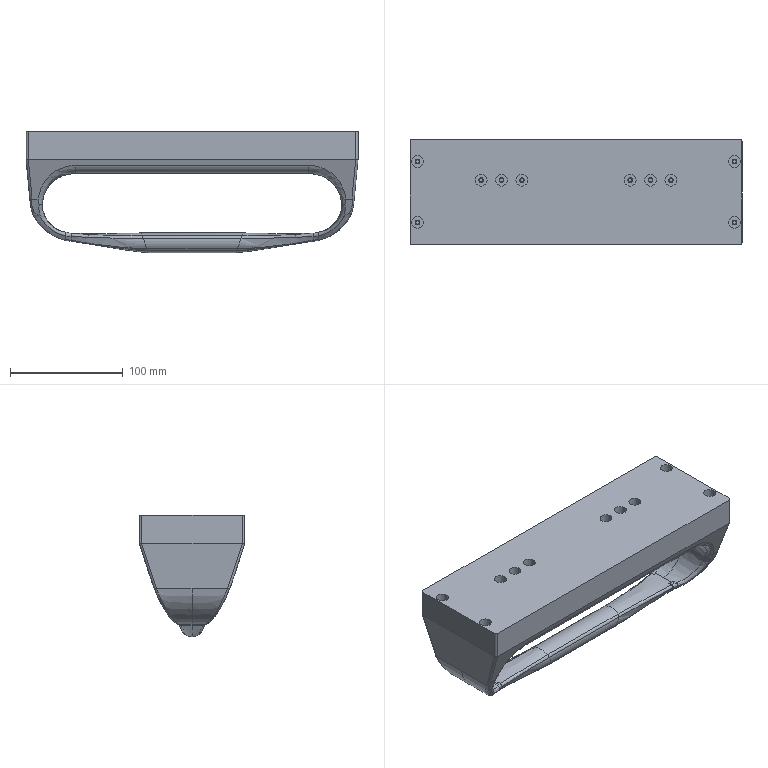NC program | NX | posted with a generic post | part box 294.078 x 93.5 x 107.5 mm
Lines 1 to 1070 of 236164:
N10 G17 G21 G94 G90
(ADAPTIVE_MILLING_COPY_COPY , TOOL : D10)
N12 T10 M6
N14 G54
N16 G17 G0 G90 X-154.596 Y2.808 B0. C0. S7500 M3
N18 G43 Z30. H10
N20 Z-14.917
N22 G94 G1 Z-15.917 F1000.
N24 X-153.005 F3000.
N26 G3 X-151.999 Y3.721 R1.015
N28 X-151.325 Y11.691 R135.716
N30 X-151.373 Y15.485 R22.541
N32 X-152.297 Y16.708 R1.622
N34 G2 X-155.294 Y21.316 R8.472
N36 X-156.13 Y27.846 R26.994
N38 X-156.226 Y46.145 R820.209
N40 G1 Y89.345
N42 X-156.225 Y89.445
N44 X-156.221 Y89.545
N46 X-156.215 Y89.645
N48 X-156.206 Y89.744
N50 G2 X-153.371 Y94.018 R6.01
N52 X-148.007 Y95.798 R12.698
N54 X-138.82 Y96.174 R78.774
N56 G1 X-137.12 Y96.18
N58 X-134.62 Y96.185
N60 X-129.82 Y96.187
N62 X149.38
N64 X149.479 Y96.184
N66 X149.579 Y96.179
N68 G2 X153.93 Y93.474 R5.901
N70 X155.842 Y87.847 R12.674
N72 X156.208 Y79.46 R73.734
N74 G1 X156.215 Y78.16
N76 X156.221 Y76.26
N78 X156.224 Y73.26
N80 X156.226 Y65.86
N82 Y24.26
N84 X156.225 Y24.16
N86 G2 X154.374 Y19.948 R6.659
N88 G3 X152.286 Y17.66 R40.145
N90 X151.571 Y15.394 R5.068
N92 X151.301 Y11.022 R47.639
N94 G1 X152.006 Y3.656
N96 G3 X152.934 Y2.745 R1.016
N98 G1 X154.705 Y2.61
N100 G2 X154.597 Y0.593 R1.01
N102 G1 Z-12.917
N104 G0 Z30.
N106 X-153.891 Y10.18
N108 Z-14.917
N110 G1 Z-15.917 F1000.
N112 G3 X-153.534 Y8.238 R-1.01 F3000.
N114 G1 X-152.715 Y8.573
N116 X-151.906 Y8.929
N118 G3 X-151.427 Y9.694 R1.025
N120 X-150.962 Y14.972 R93.028
N122 X-151.767 Y16.76 R3.073
N124 G2 X-154.951 Y25.173 R17.37
N126 X-155.395 Y34.756 R82.477
N128 G1 X-155.403 Y36.056
N130 X-155.409 Y37.856
N132 X-155.414 Y40.456
N134 X-155.417 Y44.856
N136 Y77.256
N138 Y86.556
N140 G2 X-151.732 Y92.934 R7.522
N142 X-145.405 Y94.965 R15.176
N144 X-136.118 Y95.359 R84.363
N146 G1 X-134.619 Y95.367
N148 X-132.619 Y95.373
N150 X-129.619 Y95.377
N152 X-123.119 Y95.378
N154 X146.581
N156 X146.681
N158 G2 X153.012 Y91.601 R7.583
N160 X154.987 Y85.461 R15.175
N162 X155.401 Y75.676 R85.496
N164 G1 X155.408 Y74.076
N166 X155.413 Y71.876
N168 X155.416 Y68.276
N170 X155.417 Y57.676
N172 Y26.876
N174 X155.415 Y26.676
N176 G2 X153.479 Y20.979 R10.783
N178 G3 X151.501 Y17.401 R16.875
N180 X150.929 Y14.898 R14.399
N182 G1 X151.301 Y11.016
N184 G3 X152.573 Y10.138 R1.013
N186 G1 X153.931 Y10.51
N188 G3 X153.671 Y12.494 R1.01
N190 G1 Z-12.917
N192 G0 Z30.
N194 X-153.481 Y14.462
N196 Z-14.917
N198 G1 Z-15.917 F1000.
N200 G3 X-152.887 Y12.64 R-1.01 F3000.
N202 G1 X-151.375 Y13.756
N204 G3 X-150.969 Y14.472 R1.035
N206 X-151.363 Y16.888 R3.545
N208 G2 X-154.362 Y28.83 R30.214
N210 X-154.604 Y42.125 R234.465
N212 G1 X-154.608 Y46.025
N214 X-154.609 Y57.325
N216 Y84.125
N218 X-154.606 Y84.425
N220 X-154.605 Y84.525
N222 X-154.599 Y84.725
N224 G2 X-149.8 Y92.284 R8.771
N226 X-143.007 Y94.185 R18.155
N228 X-133.018 Y94.553 R105.509
N230 G1 X-131.318 Y94.56
N232 X-129.018 Y94.565
N234 X-125.318 Y94.569
N236 X-115.618 Y94.57
N238 X-38.718
N240 X-37.718 Y94.574
N242 X-36.118 Y94.576
N244 X-34.618 Y94.575
N246 X-33.718 Y94.577
N248 X-32.818
N250 X-31.718 Y94.579
N252 X-30.718 Y94.577
N254 X-29.818 Y94.579
N256 X-28.718 Y94.577
N258 X-27.818 Y94.579
N260 X-26.818 Y94.577
N262 X-25.718 Y94.58
N264 X-24.718 Y94.578
N266 X-23.618 Y94.579
N268 X-22.818 Y94.578
N270 X-21.818 Y94.579
N272 X-20.818 Y94.578
N274 X-19.818 Y94.58
N276 X-18.718 Y94.578
N278 X-17.918 Y94.579
N280 X-16.818 Y94.577
N282 X-15.818 Y94.579
N284 X-14.918 Y94.577
N286 X-14.018 Y94.579
N288 X-13.018 Y94.577
N290 X-12.118 Y94.579
N292 X-11.218 Y94.578
N294 X-10.318 Y94.579
N296 X-9.418 Y94.578
N298 X-8.618 Y94.579
N300 X-7.618 Y94.577
N302 X-6.518 Y94.58
N304 X-5.518 Y94.578
N306 X-4.518 Y94.579
N308 X-3.018 Y94.577
N310 X-2.118 Y94.579
N312 X-1.118 Y94.578
N314 X-0.118 Y94.579
N316 X0.782 Y94.578
N318 X1.782 Y94.58
N320 X2.982 Y94.577
N322 X3.882 Y94.579
N324 X4.882 Y94.578
N326 X5.882 Y94.579
N328 X6.882 Y94.577
N330 X7.882 Y94.578
N332 X9.482 Y94.577
N334 X10.182 Y94.578
N336 X11.382 Y94.577
N338 X12.382 Y94.579
N340 X13.482 Y94.577
N342 X14.282 Y94.579
N344 X15.282 Y94.578
N346 X16.182 Y94.579
N348 X16.982 Y94.578
N350 X17.982 Y94.579
N352 X19.082 Y94.578
N354 X19.982 Y94.579
N356 X20.982 Y94.578
N358 X21.882 Y94.579
N360 X22.782 Y94.578
N362 X23.782 Y94.58
N364 X24.782 Y94.577
N366 X25.982 Y94.58
N368 X26.882 Y94.578
N370 X27.882 Y94.58
N372 X28.782 Y94.579
N374 X29.782 Y94.58
N376 X30.382
N378 X31.282 Y94.578
N380 X32.182 Y94.579
N382 X33.182 Y94.578
N384 X34.282 Y94.58
N386 X35.182 Y94.578
N388 X36.182 Y94.579
N390 X37.182 Y94.578
N392 X38.082 Y94.58
N394 X38.982 Y94.578
N396 X39.982 Y94.58
N398 X40.982 Y94.577
N400 X41.982 Y94.578
N402 X43.582 Y94.577
N404 X44.382 Y94.578
N406 X45.482 Y94.576
N408 X46.682 Y94.579
N410 X47.682 Y94.577
N412 X48.682 Y94.578
N414 X50.182 Y94.577
N416 X51.082 Y94.578
N418 X52.082 Y94.577
N420 X52.982 Y94.579
N422 X53.882 Y94.578
N424 X54.882 Y94.579
N426 X55.882 Y94.578
N428 X56.882 Y94.58
N430 X57.982 Y94.578
N432 X58.782 Y94.579
N434 X59.882 Y94.577
N436 X60.882 Y94.579
N438 X61.782 Y94.577
N440 X62.682 Y94.579
N442 X63.782 Y94.577
N444 X64.582 Y94.578
N446 X65.682 Y94.577
N448 X66.482 Y94.578
N450 X67.582 Y94.577
N452 X68.682 Y94.579
N454 X69.682 Y94.577
N456 X70.782 Y94.579
N458 X71.582 Y94.578
N460 X72.682 Y94.579
N462 X73.482 Y94.578
N464 X74.582 Y94.58
N466 X75.382 Y94.578
N468 X76.482 Y94.58
N470 X77.282 Y94.578
N472 X78.382 Y94.58
N474 X79.582 Y94.578
N476 X80.482 Y94.579
N478 X81.382 Y94.578
N480 X82.282 Y94.579
N482 X83.082 Y94.578
N484 X84.182 Y94.58
N486 X85.182 Y94.579
N488 X86.482 Y94.58
N490 X87.582 Y94.577
N492 X88.582 Y94.579
N494 X89.682 Y94.578
N496 X90.482 Y94.579
N498 X91.582 Y94.577
N500 X92.382 Y94.579
N502 X93.482 Y94.577
N504 X94.282 Y94.578
N506 X95.382 Y94.577
N508 X96.482 Y94.579
N510 X97.282 Y94.578
N512 X98.182 Y94.579
N514 X98.982 Y94.578
N516 X100.082 Y94.579
N518 X100.882 Y94.578
N520 X101.782 Y94.579
N522 X102.582 Y94.578
N524 X103.682 Y94.58
N526 X104.582 Y94.578
N528 X105.582 Y94.579
N530 X106.482 Y94.578
N532 X107.582 Y94.58
N534 X108.482 Y94.578
N536 X109.482 Y94.579
N538 X110.482 Y94.578
N540 X111.482 Y94.58
N542 X112.582 Y94.578
N544 X113.382 Y94.579
N546 X114.482 Y94.577
N548 X115.282 Y94.579
N550 X116.382 Y94.577
N552 X117.182 Y94.578
N554 X118.282 Y94.577
N556 X119.082 Y94.578
N558 X120.182 Y94.576
N560 X121.382 Y94.579
N562 X122.282 Y94.577
N564 X123.182 Y94.579
N566 X124.182 Y94.577
N568 X125.282 Y94.58
N570 X126.282 Y94.577
N572 X127.282 Y94.578
N574 X128.782 Y94.577
N576 X129.682 Y94.579
N578 X130.682 Y94.577
N580 X131.682 Y94.579
N582 X132.582 Y94.577
N584 X133.582 Y94.579
N586 X134.782 Y94.577
N588 X135.682 Y94.579
N590 X136.682 Y94.577
N592 X137.782 Y94.58
N594 X138.782 Y94.577
N596 X139.782 Y94.578
N598 X141.182 Y94.577
N600 X142.182 Y94.579
N602 G2 X146.074 Y94.432 R25.244
N604 X152.375 Y89.647 R8.904
N606 X154.224 Y82.941 R18.294
N608 X154.596 Y72.152 R113.241
N610 G1 X154.602 Y70.152
N612 X154.606 Y67.252
N614 X154.608 Y61.652
N616 X154.609 Y29.152
N618 X154.606 Y28.852
N620 X154.603 Y28.652
N622 G2 X152.746 Y21.867 R15.176
N624 G3 X150.747 Y17.08 R24.323
N626 G1 X150.737 Y16.98
N628 X150.736 Y16.913
N630 X150.937 Y14.822
N632 G3 X152.207 Y13.944 R1.013
N634 G1 X153.575 Y14.315
N636 G3 X153.306 Y16.3 R1.01
N638 G1 Z-12.917
N640 G0 Z30.
N642 X-153.404 Y15.259
N644 Z-14.917
N646 G1 Z-15.917 F1000.
N648 G3 X-152.799 Y13.438 R-1.01 F3000.
N650 G1 X-151.296 Y14.554
N652 G3 X-150.893 Y15.269 R1.035
N654 X-151.23 Y17.825 R5.93
N656 G2 X-153.655 Y32.063 R47.645
N658 X-153.8 Y54.462 R803.651
N660 G1 Y82.162
N662 X-153.798 Y82.362
N664 X-153.795 Y82.562
N666 X-153.791 Y82.762
N668 X-153.784 Y82.962
N670 X-153.775 Y83.162
N672 G2 X-148.45 Y91.403 R9.607
N674 X-141.557 Y93.33 R19.249
N676 X-131.67 Y93.737 R97.162
N678 G1 X-130.17 Y93.746
N680 X-128.47 Y93.753
N682 X-125.87 Y93.757
N684 X-121.47 Y93.76
N686 X-105.17 Y93.761
N688 X-41.47 Y93.762
N690 X-40.37 Y93.767
N692 X-39.27 Y93.768
N694 X-38.47 Y93.771
N696 X-37.47
N698 X-36.77 Y93.772
N700 X-36.27 Y93.774
N702 X-35.27
N704 X-34.27 Y93.776
N706 X-33.17
N708 X-32.07 Y93.778
N710 X-31.07 Y93.777
N712 X-29.97 Y93.779
N714 X-28.87 Y93.777
N716 X-27.87 Y93.778
N718 X-26.47 Y93.777
N720 X-25.77 Y93.778
N722 X-24.77 Y93.777
N724 X-23.87 Y93.779
N726 X-22.97 Y93.778
N728 X-21.97 Y93.779
N730 X-21.07 Y93.778
N732 X-19.97 Y93.779
N734 X-19.17 Y93.778
N736 X-18.17 Y93.779
N738 X-17.07 Y93.777
N740 X-16.07 Y93.779
N742 X-15.27 Y93.778
N744 X-14.27 Y93.779
N746 X-13.37 Y93.778
N748 X-12.47 Y93.779
N750 X-11.57 Y93.778
N752 X-10.67 Y93.779
N754 X-9.77 Y93.778
N756 X-8.77 Y93.779
N758 X-7.77 Y93.778
N760 X-6.77 Y93.779
N762 X-5.87 Y93.778
N764 X-4.67 Y93.78
N766 X-3.57 Y93.778
N768 X-2.57 Y93.779
N770 X-1.57 Y93.778
N772 X-0.47 Y93.78
N774 X0.53 Y93.778
N776 X1.73 Y93.78
N778 X2.63 Y93.778
N780 X3.63 Y93.78
N782 X4.63 Y93.778
N784 X5.53 Y93.779
N786 X6.93 Y93.776
N788 X7.93 Y93.779
N790 X9.03 Y93.777
N792 X9.93 Y93.778
N794 X10.93 Y93.777
N796 X11.93 Y93.779
N798 X12.83 Y93.777
N800 X13.93 Y93.779
N802 X14.73 Y93.778
N804 X15.73 Y93.779
N806 X16.73 Y93.778
N808 X17.63 Y93.779
N810 X18.63 Y93.777
N812 X19.63 Y93.779
N814 X20.53 Y93.778
N816 X21.53 Y93.78
N818 X22.63 Y93.778
N820 X23.63 Y93.779
N822 X24.53 Y93.778
N824 X25.53 Y93.779
N826 X26.63 Y93.778
N828 X27.83 Y93.78
N830 X28.93 Y93.778
N832 X29.73 Y93.779
N834 X30.83 Y93.778
N836 X31.93 Y93.779
N838 X32.93 Y93.778
N840 X33.83 Y93.779
N842 X34.83 Y93.778
N844 X35.93 Y93.78
N846 X36.93 Y93.778
N848 X37.73 Y93.779
N850 X38.73 Y93.778
N852 X39.93 Y93.78
N854 X40.93 Y93.777
N856 X41.93 Y93.778
N858 X42.93 Y93.777
N860 X43.53 Y93.778
N862 X44.13 Y93.779
N864 X45.33 Y93.777
N866 X46.13 Y93.778
N868 X47.13 Y93.777
N870 X48.43 Y93.78
N872 X49.53 Y93.777
N874 X50.73 Y93.78
N876 X51.63 Y93.778
N878 X52.63 Y93.779
N880 X53.63 Y93.778
N882 X54.63 Y93.779
N884 X55.73 Y93.778
N886 X56.63 Y93.779
N888 X57.53 Y93.778
N890 X58.63 Y93.779
N892 X59.63 Y93.778
N894 X60.63 Y93.779
N896 X61.63 Y93.777
N898 X62.53 Y93.778
N900 X63.63 Y93.777
N902 X64.43 Y93.778
N904 X65.63 Y93.776
N906 X66.53 Y93.778
N908 X67.53 Y93.777
N910 X68.53 Y93.779
N912 X69.43 Y93.777
N914 X70.43 Y93.779
N916 X71.33 Y93.778
N918 X72.33 Y93.78
N920 X73.23 Y93.779
N922 X74.23 Y93.78
N924 X75.13 Y93.779
N926 X76.13 Y93.78
N928 X77.23 Y93.778
N930 X78.23 Y93.779
N932 X79.13 Y93.778
N934 X80.03 Y93.779
N936 X80.93 Y93.778
N938 X81.83 Y93.78
N940 X83.03 Y93.778
N942 X84.03 Y93.78
N944 X85.13 Y93.778
N946 X86.13 Y93.779
N948 X87.23 Y93.777
N950 X88.23 Y93.779
N952 X89.13 Y93.778
N954 X90.13
N956 X91.13 Y93.777
N958 X92.13 Y93.779
N960 X93.03 Y93.777
N962 X94.13 Y93.778
N964 X95.13 Y93.777
N966 X96.03 Y93.779
N968 X97.03 Y93.777
N970 X97.93 Y93.778
N972 X99.13 Y93.777
N974 X99.93 Y93.778
N976 X101.63 Y93.775
N978 X102.13 Y93.776
N980 X102.93 Y93.778
N982 X104.13 Y93.777
N984 X105.03 Y93.779
N986 X106.13 Y93.778
N988 X107.23 Y93.78
N990 X108.13 Y93.778
N992 X109.23 Y93.78
N994 X110.23 Y93.778
N996 X111.13 Y93.779
N998 X112.23 Y93.777
N1000 X113.23 Y93.779
N1002 X114.03 Y93.777
N1004 X115.13 Y93.779
N1006 X116.13 Y93.777
N1008 X117.03 Y93.778
N1010 X117.93 Y93.777
N1012 X119.03 Y93.779
N1014 X120.03 Y93.777
N1016 X120.93 Y93.778
N1018 X121.93 Y93.777
N1020 X122.93 Y93.779
N1022 X124.03 Y93.778
N1024 X124.93 Y93.779
N1026 X126.23 Y93.776
N1028 X127.13 Y93.778
N1030 X128.33 Y93.777
N1032 X129.33 Y93.778
N1034 X130.43 Y93.777
N1036 X131.23 Y93.778
N1038 X131.93
N1040 X132.43 Y93.777
N1042 X133.43 Y93.779
N1044 X134.53 Y93.777
N1046 X135.53 Y93.779
N1048 X136.63 Y93.777
N1050 X137.53 Y93.779
N1052 X138.43 Y93.777
N1054 G2 X143.927 Y93.685 R64.834
N1056 X151.453 Y88.385 R9.631
N1058 X153.413 Y81.091 R19.746
N1060 X153.782 Y70.702 R115.958
N1062 G1 X153.789 Y69.002
N1064 X153.795 Y66.702
N1066 X153.798 Y63.102
N1068 X153.8 Y54.702
N1070 Y31.002
N1072 X153.798 Y30.802
N1074 G2 X151.996 Y22.561 R20.156
N1076 G3 X150.575 Y18.826 R34.51
N1078 G1 X150.567 Y18.726
N1080 X150.566 Y18.686
N1082 X150.738 Y16.894
N1084 G3 X152.007 Y16.016 R1.013
N1086 G1 X153.381 Y16.387
N1088 G3 X153.108 Y18.372 R1.01
N1090 G1 Z-12.917
N1092 G0 Z30.
N1094 X-153.366 Y15.657
N1096 Z-14.917
N1098 G1 Z-15.917 F1000.
N1100 G3 X-152.754 Y13.837 R-1.01 F3000.
N1102 G1 X-151.257 Y14.953
N1104 G3 X-150.855 Y15.667 R1.035
N1106 X-151.07 Y19.339 R9.924
N1108 G2 X-152.907 Y35.4 R72.288
N1110 X-152.991 Y51.199 R787.596
N1112 G1 X-152.992 Y66.399
N1114 X-152.991 Y80.199
N1116 X-152.99 Y80.499
N1118 X-152.986 Y80.799
N1120 X-152.979 Y81.099
N1122 X-152.972 Y81.299
N1124 G2 X-147.001 Y90.64 R10.334
N1126 X-139.587 Y92.556 R21.43
N1128 X-128.698 Y92.935 R121.97
N1130 G1 X-126.898 Y92.942
N1132 X-124.398 Y92.948
N1134 X-120.498 Y92.951
N1136 X-110.898 Y92.953
N1138 X-44.198
N1140 X-43.298 Y92.957
N1142 X-42.498 Y92.959
N1144 X-41.798
N1146 X-40.898 Y92.964
N1148 X-39.598 Y92.966
N1150 X-38.698 Y92.969
N1152 X-37.598
N1154 X-36.598 Y92.972
N1156 X-35.598
N1158 X-34.698 Y92.974
N1160 X-33.598
N1162 X-32.498 Y92.977
N1164 X-31.398 Y92.975
N1166 X-30.398 Y92.977
N1168 X-29.198 Y92.976
N1170 X-28.298 Y92.977
N1172 X-26.898 Y92.976
N1174 X-26.098 Y92.978
N1176 X-25.098 Y92.977
N1178 X-24.198 Y92.978
N1180 X-23.098 Y92.977
N1182 X-22.198 Y92.979
N1184 X-21.298 Y92.977
N1186 X-20.298 Y92.979
N1188 X-19.198 Y92.977
N1190 X-18.298 Y92.979
N1192 X-17.398 Y92.978
N1194 X-16.298 Y92.979
N1196 X-15.498 Y92.978
N1198 X-14.498 Y92.979
N1200 X-13.598 Y92.978
N1202 X-12.698 Y92.979
N1204 X-11.798 Y92.978
N1206 X-10.898 Y92.979
N1208 X-9.798 Y92.977
N1210 X-8.898 Y92.979
N1212 X-8.098 Y92.978
N1214 X-6.998 Y92.98
N1216 X-5.998 Y92.978
N1218 X-4.898 Y92.98
N1220 X-3.798 Y92.978
N1222 X-2.998 Y92.979
N1224 X-1.798 Y92.977
N1226 X-0.798 Y92.979
N1228 X0.102 Y92.978
N1230 X1.102 Y92.979
N1232 X2.202 Y92.978
N1234 X3.102 Y92.979
N1236 X4.302 Y92.977
N1238 X5.402 Y92.979
N1240 X6.402 Y92.977
N1242 X7.502 Y92.979
N1244 X8.502 Y92.977
N1246 X9.502 Y92.979
N1248 X10.502 Y92.977
N1250 X11.502 Y92.979
N1252 X12.402 Y92.978
N1254 X13.402 Y92.979
N1256 X14.302 Y92.978
N1258 X15.402 Y92.979
N1260 X16.502 Y92.977
N1262 X17.502 Y92.979
N1264 X18.402 Y92.978
N1266 X19.602 Y92.98
N1268 X20.502 Y92.978
N1270 X21.502 Y92.98
N1272 X22.302 Y92.978
N1274 X23.302 Y92.98
N1276 X24.302 Y92.978
N1278 X25.402 Y92.98
N1280 X26.402 Y92.979
N1282 X27.502 Y92.98
N1284 X28.502 Y92.978
N1286 X29.502 Y92.98
N1288 X30.402 Y92.979
N1290 X31.502 Y92.98
N1292 X32.602 Y92.978
N1294 X33.502 Y92.979
N1296 X34.902 Y92.978
N1298 X35.802 Y92.979
N1300 X36.702 Y92.978
N1302 X37.502 Y92.979
N1304 X38.602 Y92.978
N1306 X39.502 Y92.979
N1308 X40.602 Y92.977
N1310 X41.602 Y92.978
N1312 X42.802 Y92.977
N1314 X43.702 Y92.978
N1316 X45.002 Y92.976
N1318 X46.002 Y92.979
N1320 X47.002 Y92.978
N1322 X48.202 Y92.98
N1324 X49.302 Y92.978
N1326 X50.102 Y92.979
N1328 X51.202 Y92.977
N1330 X52.202 Y92.979
N1332 X53.202 Y92.977
N1334 X54.102 Y92.979
N1336 X55.202 Y92.977
N1338 X56.202 Y92.979
N1340 X57.202 Y92.978
N1342 X58.102 Y92.979
N1344 X59.102 Y92.978
N1346 X60.102 Y92.979
N1348 X61.202 Y92.977
N1350 X62.002 Y92.978
N1352 X63.102 Y92.977
N1354 X64.102 Y92.978
N1356 X65.102 Y92.977
N1358 X66.202 Y92.979
N1360 X67.302 Y92.977
N1362 X68.302 Y92.979
N1364 X69.302 Y92.978
N1366 X70.802 Y92.98
N1368 X71.602 Y92.979
N1370 X73.302 Y92.982
N1372 X74.502 Y92.979
N1374 X75.502 Y92.981
N1376 X76.402 Y92.979
N1378 X77.702 Y92.981
N1380 X78.602 Y92.978
N1382 X79.702 Y92.98
N1384 X80.702 Y92.978
N1386 X81.702 Y92.979
N1388 X82.802 Y92.978
N1390 X83.702 Y92.979
N1392 X84.802 Y92.978
N1394 X85.702 Y92.979
N1396 X86.902 Y92.977
N1398 X87.802 Y92.978
N1400 X89.002 Y92.977
N1402 X90.002 Y92.978
N1404 X91.002 Y92.977
N1406 X91.802 Y92.978
N1408 X92.902 Y92.977
N1410 X93.902 Y92.978
N1412 X94.802 Y92.977
N1414 X96.002 Y92.979
N1416 X96.902 Y92.977
N1418 X97.802 Y92.978
N1420 X98.702 Y92.977
N1422 X100.302 Y92.98
N1424 X101.402 Y92.978
N1426 X102.702 Y92.98
N1428 X103.202
N1430 X103.802 Y92.979
N1432 X105.002 Y92.98
N1434 X106.002 Y92.978
N1436 X106.902 Y92.98
N1438 X107.902 Y92.978
N1440 X108.802 Y92.979
N1442 X109.802 Y92.978
N1444 X110.902 Y92.979
N1446 X111.902 Y92.978
N1448 X112.902 Y92.979
N1450 X113.902 Y92.977
N1452 X114.802 Y92.979
N1454 X115.702 Y92.978
N1456 X116.802 Y92.979
N1458 X117.902 Y92.977
N1460 X118.802 Y92.979
N1462 X119.802 Y92.977
N1464 X120.702 Y92.979
N1466 X121.602 Y92.978
N1468 X122.702 Y92.979
N1470 X123.602 Y92.978
N1472 X124.802 Y92.979
N1474 X125.802 Y92.977
N1476 X126.802 Y92.978
N1478 X127.902 Y92.977
N1480 X128.902 Y92.978
N1482 X129.902 Y92.977
N1484 X131.102 Y92.979
N1486 X132.002 Y92.977
N1488 X133.102 Y92.979
N1490 X134.102 Y92.977
N1492 X135.202 Y92.979
N1494 X136.202 Y92.977
N1496 X137.302 Y92.979
N1498 X138.302 Y92.977
N1500 G2 X143.19 Y92.76 R29.1
N1502 X150.659 Y87. R10.289
N1504 X152.584 Y79.589 R21.168
N1506 X152.976 Y68. R126.652
N1508 G1 X152.983 Y66.
N1510 X152.988 Y63.3
N1512 X152.991 Y58.7
N1514 X152.992 Y41.5
N1516 Y32.8
N1518 X152.986 Y32.2
N1520 G2 X151.191 Y23.029 R25.463
N1522 G3 X150.395 Y20.662 R39.029
N1524 G1 X150.389 Y20.562
N1526 Y20.542
N1528 X150.57 Y18.651
N1530 G3 X151.839 Y17.772 R1.013
N1532 G1 X153.215 Y18.144
N1534 G3 X152.94 Y20.129 R1.01
N1536 G1 Z-12.917
N1538 G0 Z30.
N1540 X-153.28 Y16.553
N1542 Z-14.917
N1544 G1 Z-15.917 F1000.
N1546 G3 X-152.664 Y14.734 R-1.01 F3000.
N1548 G1 X-151.17 Y15.85
N1550 G3 X-150.769 Y16.563 R1.035
N1552 X-150.854 Y21.541 R15.671
N1554 G2 X-152.136 Y38.875 R111.031
N1556 G1 X-152.148 Y40.075
N1558 X-152.159 Y41.475
N1560 X-152.167 Y43.175
N1562 X-152.174 Y45.475
N1564 X-152.179 Y48.575
N1566 X-152.182 Y53.775
N1568 X-152.183 Y74.875
N1570 Y78.475
N1572 X-152.177 Y79.075
N1574 X-152.174 Y79.275
N1576 X-152.163 Y79.675
N1578 G2 X-149.628 Y86.881 R11.157
N1580 X-142.946 Y90.876 R13.398
N1582 X-134.737 Y91.975 R36.695
N1584 X-119.139 Y92.142 R434.152
N1586 G1 X-111.539 Y92.144
N1588 X-46.939 Y92.145
N1590 X-46.039 Y92.149
N1592 X-45.239 Y92.15
N1594 X-44.539
N1596 X-43.239 Y92.157
N1598 X-42.339 Y92.158
N1600 X-41.239 Y92.163
N1602 X-40.139 Y92.164
N1604 X-39.139 Y92.167
N1606 X-37.939
N1608 X-37.139 Y92.17
N1610 X-35.939
N1612 X-34.939 Y92.173
N1614 X-33.739
N1616 X-32.639 Y92.176
N1618 X-31.439 Y92.174
N1620 X-30.539 Y92.177
N1622 X-29.439 Y92.175
N1624 X-28.439 Y92.176
N1626 X-27.439 Y92.175
N1628 X-26.439 Y92.177
N1630 X-25.439 Y92.176
N1632 X-24.439 Y92.178
N1634 X-23.339 Y92.176
N1636 X-22.439 Y92.178
N1638 X-21.439 Y92.177
N1640 X-20.539 Y92.178
N1642 X-19.439 Y92.177
N1644 X-18.439 Y92.179
N1646 X-17.639 Y92.178
N1648 X-16.639 Y92.179
N1650 X-15.739 Y92.178
N1652 X-14.739 Y92.18
N1654 X-13.639 Y92.178
N1656 X-12.839 Y92.179
N1658 X-11.739 Y92.177
N1660 X-10.939 Y92.178
N1662 X-10.039 Y92.177
N1664 X-9.039 Y92.179
N1666 X-8.139 Y92.178
N1668 X-7.139 Y92.179
N1670 X-6.039 Y92.178
N1672 X-5.139 Y92.179
N1674 X-4.039 Y92.177
N1676 X-2.939 Y92.179
N1678 X-1.939 Y92.178
N1680 X-1.039 Y92.179
N1682 X-0.139 Y92.178
N1684 X0.961 Y92.179
N1686 X1.861 Y92.178
N1688 X3.061 Y92.179
N1690 X4.06 Y92.177
N1692 X5.16 Y92.179
N1694 X6.26 Y92.177
N1696 X7.26 Y92.178
N1698 X8.26 Y92.177
N1700 X9.26 Y92.178
N1702 X10.26 Y92.177
N1704 X11.26 Y92.179
N1706 X12.36 Y92.177
N1708 X13.26 Y92.179
N1710 X14.26 Y92.178
N1712 X15.26 Y92.179
N1714 X16.26 Y92.178
N1716 X17.16 Y92.179
N1718 X18.26 Y92.178
N1720 X19.26 Y92.179
N1722 X20.16 Y92.178
N1724 X21.16 Y92.18
N1726 X22.16 Y92.178
N1728 X23.16 Y92.18
N1730 X24.06 Y92.178
N1732 X25.06 Y92.18
N1734 X26.26 Y92.178
N1736 X27.26 Y92.18
N1738 X28.16 Y92.178
N1740 X29.26 Y92.18
N1742 X30.26 Y92.179
N1744 X31.36 Y92.18
N1746 X32.46 Y92.178
N1748 X33.46 Y92.179
N1750 X34.46 Y92.178
N1752 X35.56 Y92.179
N1754 X36.56 Y92.178
N1756 X37.46 Y92.179
N1758 X38.36 Y92.178
N1760 X39.46 Y92.179
N1762 X40.36 Y92.178
N1764 X41.66 Y92.179
N1766 X42.46 Y92.178
N1768 X43.16
N1770 X43.76 Y92.179
N1772 X44.66 Y92.178
N1774 X45.76 Y92.179
N1776 X46.86 Y92.177
N1778 X47.86 Y92.179
N1780 X48.76 Y92.178
N1782 X49.86 Y92.179
N1784 X50.96 Y92.177
N1786 X52.06 Y92.179
N1788 X52.96 Y92.178
N1790 X54.26 Y92.179
N1792 X55.06 Y92.178
N1794 X55.96 Y92.179
N1796 X57.06 Y92.178
N1798 X57.86 Y92.179
N1800 X58.96 Y92.177
N1802 X59.86 Y92.178
N1804 X60.86 Y92.177
N1806 X61.86 Y92.178
N1808 X62.96 Y92.176
N1810 X63.96 Y92.178
N1812 X64.96 Y92.177
N1814 X66.06 Y92.179
N1816 X67.16 Y92.177
N1818 X68.16 Y92.179
N1820 X69.16 Y92.178
N1822 X69.66 Y92.179
N1824 X70.56 Y92.182
N1826 X71.86 Y92.179
N1828 X72.86 Y92.181
N1830 X73.86 Y92.179
N1832 X74.76 Y92.18
N1834 X76.06 Y92.178
N1836 X76.86 Y92.179
N1838 X77.46
N1840 X78.06 Y92.177
N1842 X79.16 Y92.179
N1844 X80.56 Y92.177
N1846 X81.46 Y92.178
N1848 X82.76 Y92.177
N1850 X83.66 Y92.178
N1852 X84.76 Y92.177
N1854 X85.66 Y92.178
N1856 X86.66 Y92.177
N1858 X87.66 Y92.178
N1860 X88.76 Y92.177
N1862 X89.76 Y92.179
N1864 X90.66 Y92.177
N1866 X91.76 Y92.178
N1868 X92.76 Y92.177
N1870 X93.76 Y92.179
N1872 X94.76 Y92.177
N1874 X95.66 Y92.178
N1876 X96.66 Y92.177
N1878 X97.86 Y92.179
N1880 X98.86 Y92.178
N1882 X100.26 Y92.181
N1884 X101.26 Y92.179
N1886 X102.46 Y92.181
N1888 X103.36 Y92.179
N1890 X104.56 Y92.181
N1892 X105.66 Y92.178
N1894 X106.46 Y92.18
N1896 X107.56 Y92.178
N1898 X108.46 Y92.179
N1900 X109.56 Y92.178
N1902 X110.66 Y92.179
N1904 X111.66 Y92.178
N1906 X112.56 Y92.179
N1908 X113.56 Y92.178
N1910 X114.46 Y92.179
N1912 X115.56 Y92.177
N1914 X116.56 Y92.179
N1916 X117.56 Y92.177
N1918 X118.56 Y92.179
N1920 X119.46 Y92.178
N1922 X120.46 Y92.179
N1924 X121.56 Y92.178
N1926 X122.56 Y92.179
N1928 X123.56 Y92.177
N1930 X124.46 Y92.178
N1932 X125.56 Y92.177
N1934 G2 X140.06 Y92.133 R780.406
N1936 X149.917 Y85.589 R10.943
N1938 X151.787 Y77.953 R23.146
N1940 X152.169 Y65.563 R144.77
N1942 G1 X152.175 Y63.363
N1944 X152.18 Y60.263
N1946 X152.182 Y54.663
N1948 X152.183 Y34.363
N1950 X152.179 Y33.663
N1952 X152.17 Y33.163
N1954 G2 X150.375 Y23.37 R31.453
N1956 G3 X150.193 Y22.586 R8.412
N1958 G1 X150.393 Y20.496
N1960 G3 X151.662 Y19.617 R1.013
N1962 G1 X153.039 Y19.989
N1964 G3 X152.763 Y21.974 R1.01
N1966 G1 Z-12.917
N1968 G0 Z30.
N1970 X-153.128 Y18.146
N1972 Z-14.917
N1974 G1 Z-15.917 F1000.
N1976 G3 X-152.511 Y16.327 R-1.01 F3000.
N1978 G1 X-151.017 Y17.443
N1980 G3 X-150.617 Y18.155 R1.035
N1982 X-150.601 Y25.035 R25.954
N1984 G2 X-151.347 Y42.112 R175.918
N1986 G1 X-151.355 Y43.512
N1988 X-151.363 Y45.612
N1990 X-151.369 Y48.512
N1992 X-151.373 Y52.812
N1994 X-151.374 Y62.012
N1996 Y76.812
N1998 G2 X-150.731 Y82.25 R17.619
N2000 X-144.39 Y89.078 R11.423
N2002 X-136.447 Y90.951 R24.327
N2004 X-124.257 Y91.32 R149.591
N2006 G1 X-122.057 Y91.327
N2008 X-119.257 Y91.332
N2010 X-114.357 Y91.335
N2012 X-95.257 Y91.336
N2014 X-49.657
N2016 X-48.757 Y91.34
N2018 X-47.657 Y91.341
N2020 X-47.157 Y91.342
N2022 X-45.857 Y91.349
N2024 X-44.757 Y91.35
N2026 X-43.657 Y91.356
N2028 X-42.557 Y91.357
N2030 X-41.557 Y91.361
N2032 X-40.357 Y91.362
N2034 X-39.457 Y91.365
N2036 X-38.357 Y91.366
N2038 X-37.657 Y91.367
N2040 X-37.057 Y91.37
N2042 X-36.057 Y91.369
N2044 X-35.057 Y91.372
N2046 X-34.357
N2048 X-33.757 Y91.371
N2050 X-32.957 Y91.374
N2052 X-32.257 Y91.373
N2054 X-31.657
N2056 X-30.857 Y91.375
N2058 X-29.757 Y91.374
N2060 X-28.857 Y91.376
N2062 X-27.757 Y91.375
N2064 X-26.857 Y91.376
N2066 X-25.757 Y91.375
N2068 X-24.857 Y91.377
N2070 X-23.757 Y91.376
N2072 X-22.857 Y91.377
N2074 X-21.757 Y91.376
N2076 X-20.857 Y91.378
N2078 X-19.657 Y91.376
N2080 X-18.757 Y91.378
N2082 X-17.857 Y91.377
N2084 X-16.857 Y91.379
N2086 X-15.857 Y91.377
N2088 X-14.857 Y91.379
N2090 X-13.857 Y91.377
N2092 X-12.957 Y91.378
N2094 X-11.957 Y91.377
N2096 X-11.057 Y91.378
N2098 X-10.157 Y91.377
N2100 X-9.257 Y91.379
N2102 X-8.157 Y91.377
N2104 X-7.357 Y91.379
N2106 X-6.357 Y91.378
N2108 X-5.257 Y91.379
N2110 X-4.157 Y91.378
N2112 X-3.057 Y91.379
N2114 X-2.157 Y91.378
N2116 X-1.157 Y91.379
N2118 X-0.257 Y91.378
N2120 X0.743 Y91.379
N2122 X1.943 Y91.377
N2124 X2.843 Y91.379
N2126 X3.943 Y91.377
N2128 X4.843 Y91.378
N2130 X5.943 Y91.377
N2132 X6.843 Y91.378
N2134 X8.043 Y91.376
N2136 X9.043 Y91.378
N2138 X10.143 Y91.377